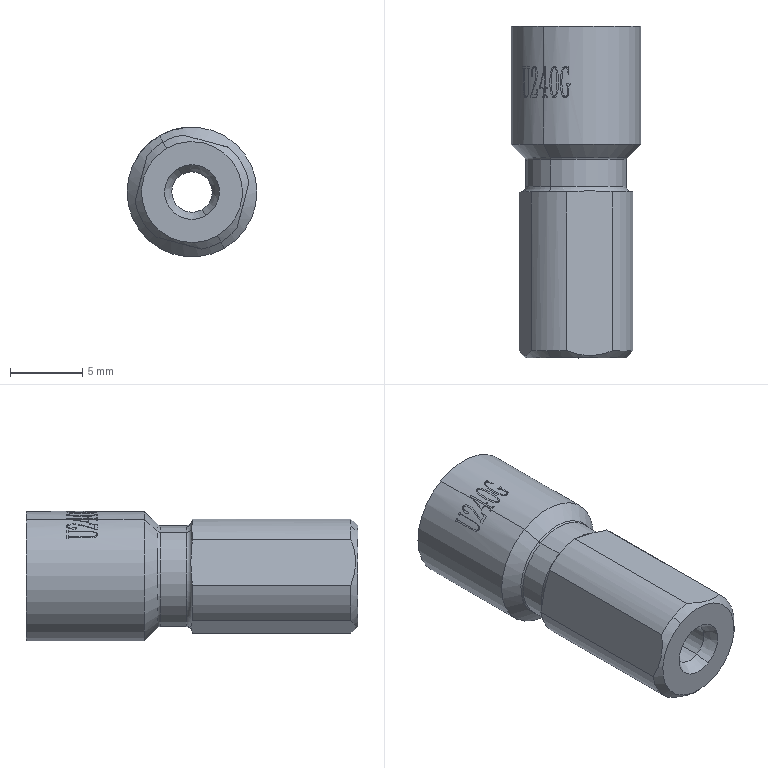Part | SolidWorks | features BaseBody 1 | 1 solid | 53 faces | box 9 x 23 x 9 mm | volume 856.218 mm3 | cylinder 25 | plane 12 | cone 10 | torus 6 | commonest cylinder face diameters 9 x10 8 x5 2.8 x2 5 x2 5.2 x2 5.7 x2